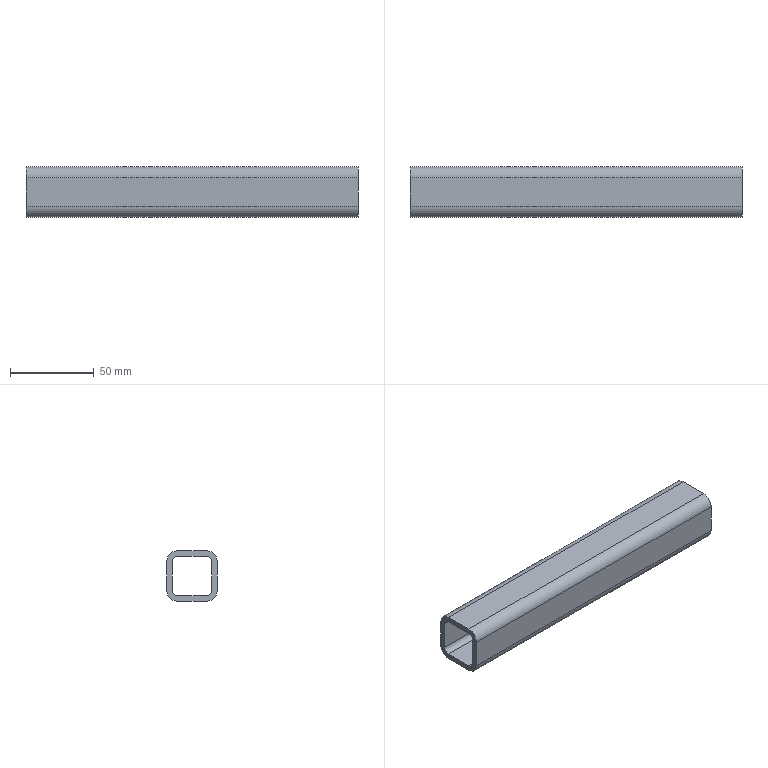Part | STEP file | [01]-7 | 1 solid | 18 faces | box 197.8 x 30 x 30 mm | volume 62637 mm3 | plane 10 | cylinder 8 | commonest cylinder face diameters 6.4 x4 12.8 x4
STEP:
#1=CARTESIAN_POINT('',(5.,23.6,0.));
#2=VERTEX_POINT('',#1);
#3=CARTESIAN_POINT('',(5.,30.,6.4));
#4=VERTEX_POINT('',#3);
#5=CARTESIAN_POINT('',(5.,23.6,6.4));
#6=DIRECTION('',(1.,0.,0.));
#7=DIRECTION('',(0.,0.,-1.));
#8=AXIS2_PLACEMENT_3D('',#5,#6,#7);
#9=CIRCLE('',#8,6.4);
#10=EDGE_CURVE('',#2,#4,#9,.T.);
#11=ORIENTED_EDGE('',*,*,#10,.T.);
#12=CARTESIAN_POINT('',(202.8,30.,6.4));
#13=VERTEX_POINT('',#12);
#14=CARTESIAN_POINT('',(202.8,30.,6.4));
#15=DIRECTION('',(-1.,0.,0.));
#16=VECTOR('',#15,1000.);
#17=LINE('',#14,#16);
#18=EDGE_CURVE('',#13,#4,#17,.T.);
#19=ORIENTED_EDGE('',*,*,#18,.F.);
#20=CARTESIAN_POINT('',(202.8,23.6,0.));
#21=VERTEX_POINT('',#20);
#22=CARTESIAN_POINT('',(202.8,23.6,6.4));
#23=DIRECTION('',(1.,0.,0.));
#24=DIRECTION('',(0.,0.,-1.));
#25=AXIS2_PLACEMENT_3D('',#22,#23,#24);
#26=CIRCLE('',#25,6.4);
#27=EDGE_CURVE('',#21,#13,#26,.T.);
#28=ORIENTED_EDGE('',*,*,#27,.F.);
#29=CARTESIAN_POINT('',(202.8,23.6,0.));
#30=DIRECTION('',(-1.,0.,0.));
#31=VECTOR('',#30,1000.);
#32=LINE('',#29,#31);
#33=EDGE_CURVE('',#21,#2,#32,.T.);
#34=ORIENTED_EDGE('',*,*,#33,.T.);
#35=EDGE_LOOP('',(#11,#19,#28,#34));
#36=FACE_OUTER_BOUND('',#35,.T.);
#37=CARTESIAN_POINT('',(202.8,23.6,6.4));
#38=DIRECTION('',(-1.,0.,0.));
#39=DIRECTION('',(0.,0.,1.));
#40=AXIS2_PLACEMENT_3D('',#37,#38,#39);
#41=CYLINDRICAL_SURFACE('',#40,6.4);
#42=ADVANCED_FACE('',(#36),#41,.T.);
#43=CARTESIAN_POINT('',(5.,30.,23.6));
#44=VERTEX_POINT('',#43);
#45=CARTESIAN_POINT('',(5.,30.,6.4));
#46=DIRECTION('',(0.,0.,1.));
#47=VECTOR('',#46,1000.);
#48=LINE('',#45,#47);
#49=EDGE_CURVE('',#4,#44,#48,.T.);
#50=ORIENTED_EDGE('',*,*,#49,.T.);
#51=CARTESIAN_POINT('',(202.8,30.,23.6));
#52=VERTEX_POINT('',#51);
#53=CARTESIAN_POINT('',(202.8,30.,23.6));
#54=DIRECTION('',(-1.,0.,0.));
#55=VECTOR('',#54,1000.);
#56=LINE('',#53,#55);
#57=EDGE_CURVE('',#52,#44,#56,.T.);
#58=ORIENTED_EDGE('',*,*,#57,.F.);
#59=CARTESIAN_POINT('',(202.8,30.,6.4));
#60=DIRECTION('',(0.,0.,1.));
#61=VECTOR('',#60,1000.);
#62=LINE('',#59,#61);
#63=EDGE_CURVE('',#13,#52,#62,.T.);
#64=ORIENTED_EDGE('',*,*,#63,.F.);
#65=ORIENTED_EDGE('',*,*,#18,.T.);
#66=EDGE_LOOP('',(#50,#58,#64,#65));
#67=FACE_OUTER_BOUND('',#66,.T.);
#68=CARTESIAN_POINT('',(202.8,30.,6.4));
#69=DIRECTION('',(0.,-1.,0.));
#70=DIRECTION('',(0.,0.,-1.));
#71=AXIS2_PLACEMENT_3D('',#68,#69,#70);
#72=PLANE('',#71);
#73=ADVANCED_FACE('',(#67),#72,.F.);
#74=CARTESIAN_POINT('',(5.,23.6,30.));
#75=VERTEX_POINT('',#74);
#76=CARTESIAN_POINT('',(5.,23.6,23.6));
#77=DIRECTION('',(1.,0.,0.));
#78=DIRECTION('',(0.,0.,-1.));
#79=AXIS2_PLACEMENT_3D('',#76,#77,#78);
#80=CIRCLE('',#79,6.4);
#81=EDGE_CURVE('',#44,#75,#80,.T.);
#82=ORIENTED_EDGE('',*,*,#81,.T.);
#83=CARTESIAN_POINT('',(202.8,23.6,30.));
#84=VERTEX_POINT('',#83);
#85=CARTESIAN_POINT('',(202.8,23.6,30.));
#86=DIRECTION('',(-1.,0.,0.));
#87=VECTOR('',#86,1000.);
#88=LINE('',#85,#87);
#89=EDGE_CURVE('',#84,#75,#88,.T.);
#90=ORIENTED_EDGE('',*,*,#89,.F.);
#91=CARTESIAN_POINT('',(202.8,23.6,23.6));
#92=DIRECTION('',(1.,0.,0.));
#93=DIRECTION('',(0.,0.,-1.));
#94=AXIS2_PLACEMENT_3D('',#91,#92,#93);
#95=CIRCLE('',#94,6.4);
#96=EDGE_CURVE('',#52,#84,#95,.T.);
#97=ORIENTED_EDGE('',*,*,#96,.F.);
#98=ORIENTED_EDGE('',*,*,#57,.T.);
#99=EDGE_LOOP('',(#82,#90,#97,#98));
#100=FACE_OUTER_BOUND('',#99,.T.);
#101=CARTESIAN_POINT('',(202.8,23.6,23.6));
#102=DIRECTION('',(-1.,0.,0.));
#103=DIRECTION('',(0.,0.,1.));
#104=AXIS2_PLACEMENT_3D('',#101,#102,#103);
#105=CYLINDRICAL_SURFACE('',#104,6.4);
#106=ADVANCED_FACE('',(#100),#105,.T.);
#107=CARTESIAN_POINT('',(5.,6.4,30.));
#108=VERTEX_POINT('',#107);
#109=CARTESIAN_POINT('',(5.,23.6,30.));
#110=DIRECTION('',(0.,-1.,0.));
#111=VECTOR('',#110,1000.);
#112=LINE('',#109,#111);
#113=EDGE_CURVE('',#75,#108,#112,.T.);
#114=ORIENTED_EDGE('',*,*,#113,.T.);
#115=CARTESIAN_POINT('',(202.8,6.4,30.));
#116=VERTEX_POINT('',#115);
#117=CARTESIAN_POINT('',(202.8,6.4,30.));
#118=DIRECTION('',(-1.,0.,0.));
#119=VECTOR('',#118,1000.);
#120=LINE('',#117,#119);
#121=EDGE_CURVE('',#116,#108,#120,.T.);
#122=ORIENTED_EDGE('',*,*,#121,.F.);
#123=CARTESIAN_POINT('',(202.8,23.6,30.));
#124=DIRECTION('',(0.,-1.,0.));
#125=VECTOR('',#124,1000.);
#126=LINE('',#123,#125);
#127=EDGE_CURVE('',#84,#116,#126,.T.);
#128=ORIENTED_EDGE('',*,*,#127,.F.);
#129=ORIENTED_EDGE('',*,*,#89,.T.);
#130=EDGE_LOOP('',(#114,#122,#128,#129));
#131=FACE_OUTER_BOUND('',#130,.T.);
#132=CARTESIAN_POINT('',(202.8,23.6,30.));
#133=DIRECTION('',(0.,0.,-1.));
#134=DIRECTION('',(0.,1.,0.));
#135=AXIS2_PLACEMENT_3D('',#132,#133,#134);
#136=PLANE('',#135);
#137=ADVANCED_FACE('',(#131),#136,.F.);
#138=CARTESIAN_POINT('',(5.,0.,23.6));
#139=VERTEX_POINT('',#138);
#140=CARTESIAN_POINT('',(5.,6.4,23.6));
#141=DIRECTION('',(1.,0.,0.));
#142=DIRECTION('',(0.,0.,-1.));
#143=AXIS2_PLACEMENT_3D('',#140,#141,#142);
#144=CIRCLE('',#143,6.4);
#145=EDGE_CURVE('',#108,#139,#144,.T.);
#146=ORIENTED_EDGE('',*,*,#145,.T.);
#147=CARTESIAN_POINT('',(202.8,0.,23.6));
#148=VERTEX_POINT('',#147);
#149=CARTESIAN_POINT('',(202.8,0.,23.6));
#150=DIRECTION('',(-1.,0.,0.));
#151=VECTOR('',#150,1000.);
#152=LINE('',#149,#151);
#153=EDGE_CURVE('',#148,#139,#152,.T.);
#154=ORIENTED_EDGE('',*,*,#153,.F.);
#155=CARTESIAN_POINT('',(202.8,6.4,23.6));
#156=DIRECTION('',(1.,0.,0.));
#157=DIRECTION('',(0.,0.,-1.));
#158=AXIS2_PLACEMENT_3D('',#155,#156,#157);
#159=CIRCLE('',#158,6.4);
#160=EDGE_CURVE('',#116,#148,#159,.T.);
#161=ORIENTED_EDGE('',*,*,#160,.F.);
#162=ORIENTED_EDGE('',*,*,#121,.T.);
#163=EDGE_LOOP('',(#146,#154,#161,#162));
#164=FACE_OUTER_BOUND('',#163,.T.);
#165=CARTESIAN_POINT('',(202.8,6.4,23.6));
#166=DIRECTION('',(-1.,0.,0.));
#167=DIRECTION('',(0.,0.,1.));
#168=AXIS2_PLACEMENT_3D('',#165,#166,#167);
#169=CYLINDRICAL_SURFACE('',#168,6.4);
#170=ADVANCED_FACE('',(#164),#169,.T.);
#171=CARTESIAN_POINT('',(5.,0.,6.4));
#172=VERTEX_POINT('',#171);
#173=CARTESIAN_POINT('',(5.,0.,23.6));
#174=DIRECTION('',(0.,0.,-1.));
#175=VECTOR('',#174,1000.);
#176=LINE('',#173,#175);
#177=EDGE_CURVE('',#139,#172,#176,.T.);
#178=ORIENTED_EDGE('',*,*,#177,.T.);
#179=CARTESIAN_POINT('',(202.8,0.,6.4));
#180=VERTEX_POINT('',#179);
#181=CARTESIAN_POINT('',(202.8,0.,6.4));
#182=DIRECTION('',(-1.,0.,0.));
#183=VECTOR('',#182,1000.);
#184=LINE('',#181,#183);
#185=EDGE_CURVE('',#180,#172,#184,.T.);
#186=ORIENTED_EDGE('',*,*,#185,.F.);
#187=CARTESIAN_POINT('',(202.8,0.,23.6));
#188=DIRECTION('',(0.,0.,-1.));
#189=VECTOR('',#188,1000.);
#190=LINE('',#187,#189);
#191=EDGE_CURVE('',#148,#180,#190,.T.);
#192=ORIENTED_EDGE('',*,*,#191,.F.);
#193=ORIENTED_EDGE('',*,*,#153,.T.);
#194=EDGE_LOOP('',(#178,#186,#192,#193));
#195=FACE_OUTER_BOUND('',#194,.T.);
#196=CARTESIAN_POINT('',(202.8,0.,23.6));
#197=DIRECTION('',(0.,1.,0.));
#198=DIRECTION('',(0.,0.,1.));
#199=AXIS2_PLACEMENT_3D('',#196,#197,#198);
#200=PLANE('',#199);
#201=ADVANCED_FACE('',(#195),#200,.F.);
#202=CARTESIAN_POINT('',(5.,6.4,0.));
#203=VERTEX_POINT('',#202);
#204=CARTESIAN_POINT('',(5.,6.4,6.4));
#205=DIRECTION('',(1.,0.,0.));
#206=DIRECTION('',(0.,0.,-1.));
#207=AXIS2_PLACEMENT_3D('',#204,#205,#206);
#208=CIRCLE('',#207,6.4);
#209=EDGE_CURVE('',#172,#203,#208,.T.);
#210=ORIENTED_EDGE('',*,*,#209,.T.);
#211=CARTESIAN_POINT('',(202.8,6.4,0.));
#212=VERTEX_POINT('',#211);
#213=CARTESIAN_POINT('',(202.8,6.4,0.));
#214=DIRECTION('',(-1.,0.,0.));
#215=VECTOR('',#214,1000.);
#216=LINE('',#213,#215);
#217=EDGE_CURVE('',#212,#203,#216,.T.);
#218=ORIENTED_EDGE('',*,*,#217,.F.);
#219=CARTESIAN_POINT('',(202.8,6.4,6.4));
#220=DIRECTION('',(1.,0.,0.));
#221=DIRECTION('',(0.,0.,-1.));
#222=AXIS2_PLACEMENT_3D('',#219,#220,#221);
#223=CIRCLE('',#222,6.4);
#224=EDGE_CURVE('',#180,#212,#223,.T.);
#225=ORIENTED_EDGE('',*,*,#224,.F.);
#226=ORIENTED_EDGE('',*,*,#185,.T.);
#227=EDGE_LOOP('',(#210,#218,#225,#226));
#228=FACE_OUTER_BOUND('',#227,.T.);
#229=CARTESIAN_POINT('',(202.8,6.4,6.4));
#230=DIRECTION('',(-1.,0.,0.));
#231=DIRECTION('',(0.,0.,1.));
#232=AXIS2_PLACEMENT_3D('',#229,#230,#231);
#233=CYLINDRICAL_SURFACE('',#232,6.4);
#234=ADVANCED_FACE('',(#228),#233,.T.);
#235=CARTESIAN_POINT('',(5.,6.4,0.));
#236=DIRECTION('',(0.,1.,0.));
#237=VECTOR('',#236,1000.);
#238=LINE('',#235,#237);
#239=EDGE_CURVE('',#203,#2,#238,.T.);
#240=ORIENTED_EDGE('',*,*,#239,.T.);
#241=ORIENTED_EDGE('',*,*,#33,.F.);
#242=CARTESIAN_POINT('',(202.8,6.4,0.));
#243=DIRECTION('',(0.,1.,0.));
#244=VECTOR('',#243,1000.);
#245=LINE('',#242,#244);
#246=EDGE_CURVE('',#212,#21,#245,.T.);
#247=ORIENTED_EDGE('',*,*,#246,.F.);
#248=ORIENTED_EDGE('',*,*,#217,.T.);
#249=EDGE_LOOP('',(#240,#241,#247,#248));
#250=FACE_OUTER_BOUND('',#249,.T.);
#251=CARTESIAN_POINT('',(202.8,6.4,0.));
#252=DIRECTION('',(0.,0.,1.));
#253=DIRECTION('',(0.,-1.,0.));
#254=AXIS2_PLACEMENT_3D('',#251,#252,#253);
#255=PLANE('',#254);
#256=ADVANCED_FACE('',(#250),#255,.F.);
#257=CARTESIAN_POINT('',(202.8,26.8,23.6));
#258=VERTEX_POINT('',#257);
#259=CARTESIAN_POINT('',(202.8,23.6,26.8));
#260=VERTEX_POINT('',#259);
#261=CARTESIAN_POINT('',(202.8,23.6,23.6));
#262=DIRECTION('',(1.,0.,0.));
#263=DIRECTION('',(0.,0.,-1.));
#264=AXIS2_PLACEMENT_3D('',#261,#262,#263);
#265=CIRCLE('',#264,3.2);
#266=EDGE_CURVE('',#258,#260,#265,.T.);
#267=ORIENTED_EDGE('',*,*,#266,.F.);
#268=CARTESIAN_POINT('',(202.8,26.8,6.4));
#269=VERTEX_POINT('',#268);
#270=CARTESIAN_POINT('',(202.8,26.8,6.4));
#271=DIRECTION('',(0.,0.,1.));
#272=VECTOR('',#271,1000.);
#273=LINE('',#270,#272);
#274=EDGE_CURVE('',#269,#258,#273,.T.);
#275=ORIENTED_EDGE('',*,*,#274,.F.);
#276=CARTESIAN_POINT('',(202.8,23.6,3.2));
#277=VERTEX_POINT('',#276);
#278=CARTESIAN_POINT('',(202.8,23.6,6.4));
#279=DIRECTION('',(1.,0.,0.));
#280=DIRECTION('',(0.,0.,-1.));
#281=AXIS2_PLACEMENT_3D('',#278,#279,#280);
#282=CIRCLE('',#281,3.2);
#283=EDGE_CURVE('',#277,#269,#282,.T.);
#284=ORIENTED_EDGE('',*,*,#283,.F.);
#285=CARTESIAN_POINT('',(202.8,6.4,3.2));
#286=VERTEX_POINT('',#285);
#287=CARTESIAN_POINT('',(202.8,6.4,3.2));
#288=DIRECTION('',(0.,1.,0.));
#289=VECTOR('',#288,1000.);
#290=LINE('',#287,#289);
#291=EDGE_CURVE('',#286,#277,#290,.T.);
#292=ORIENTED_EDGE('',*,*,#291,.F.);
#293=CARTESIAN_POINT('',(202.8,3.2,6.4));
#294=VERTEX_POINT('',#293);
#295=CARTESIAN_POINT('',(202.8,6.4,6.4));
#296=DIRECTION('',(1.,0.,0.));
#297=DIRECTION('',(0.,0.,-1.));
#298=AXIS2_PLACEMENT_3D('',#295,#296,#297);
#299=CIRCLE('',#298,3.2);
#300=EDGE_CURVE('',#294,#286,#299,.T.);
#301=ORIENTED_EDGE('',*,*,#300,.F.);
#302=CARTESIAN_POINT('',(202.8,3.2,23.6));
#303=VERTEX_POINT('',#302);
#304=CARTESIAN_POINT('',(202.8,3.2,23.6));
#305=DIRECTION('',(0.,0.,-1.));
#306=VECTOR('',#305,1000.);
#307=LINE('',#304,#306);
#308=EDGE_CURVE('',#303,#294,#307,.T.);
#309=ORIENTED_EDGE('',*,*,#308,.F.);
#310=CARTESIAN_POINT('',(202.8,6.4,26.8));
#311=VERTEX_POINT('',#310);
#312=CARTESIAN_POINT('',(202.8,6.4,23.6));
#313=DIRECTION('',(1.,0.,0.));
#314=DIRECTION('',(0.,0.,-1.));
#315=AXIS2_PLACEMENT_3D('',#312,#313,#314);
#316=CIRCLE('',#315,3.2);
#317=EDGE_CURVE('',#311,#303,#316,.T.);
#318=ORIENTED_EDGE('',*,*,#317,.F.);
#319=CARTESIAN_POINT('',(202.8,23.6,26.8));
#320=DIRECTION('',(0.,-1.,0.));
#321=VECTOR('',#320,1000.);
#322=LINE('',#319,#321);
#323=EDGE_CURVE('',#260,#311,#322,.T.);
#324=ORIENTED_EDGE('',*,*,#323,.F.);
#325=EDGE_LOOP('',(#267,#275,#284,#292,#301,#309,#318,#324));
#326=FACE_BOUND('',#325,.T.);
#327=ORIENTED_EDGE('',*,*,#27,.T.);
#328=ORIENTED_EDGE('',*,*,#63,.T.);
#329=ORIENTED_EDGE('',*,*,#96,.T.);
#330=ORIENTED_EDGE('',*,*,#127,.T.);
#331=ORIENTED_EDGE('',*,*,#160,.T.);
#332=ORIENTED_EDGE('',*,*,#191,.T.);
#333=ORIENTED_EDGE('',*,*,#224,.T.);
#334=ORIENTED_EDGE('',*,*,#246,.T.);
#335=EDGE_LOOP('',(#327,#328,#329,#330,#331,#332,#333,#334));
#336=FACE_OUTER_BOUND('',#335,.T.);
#337=CARTESIAN_POINT('',(202.8,23.6,6.4));
#338=DIRECTION('',(1.,0.,0.));
#339=DIRECTION('',(0.,0.,-1.));
#340=AXIS2_PLACEMENT_3D('',#337,#338,#339);
#341=PLANE('',#340);
#342=ADVANCED_FACE('',(#326,#336),#341,.T.);
#343=CARTESIAN_POINT('',(5.,26.8,6.4));
#344=VERTEX_POINT('',#343);
#345=CARTESIAN_POINT('',(5.,26.8,23.6));
#346=VERTEX_POINT('',#345);
#347=CARTESIAN_POINT('',(5.,26.8,6.4));
#348=DIRECTION('',(0.,0.,1.));
#349=VECTOR('',#348,1000.);
#350=LINE('',#347,#349);
#351=EDGE_CURVE('',#344,#346,#350,.T.);
#352=ORIENTED_EDGE('',*,*,#351,.T.);
#353=CARTESIAN_POINT('',(5.,23.6,26.8));
#354=VERTEX_POINT('',#353);
#355=CARTESIAN_POINT('',(5.,23.6,23.6));
#356=DIRECTION('',(1.,0.,0.));
#357=DIRECTION('',(0.,0.,-1.));
#358=AXIS2_PLACEMENT_3D('',#355,#356,#357);
#359=CIRCLE('',#358,3.2);
#360=EDGE_CURVE('',#346,#354,#359,.T.);
#361=ORIENTED_EDGE('',*,*,#360,.T.);
#362=CARTESIAN_POINT('',(5.,6.4,26.8));
#363=VERTEX_POINT('',#362);
#364=CARTESIAN_POINT('',(5.,23.6,26.8));
#365=DIRECTION('',(0.,-1.,0.));
#366=VECTOR('',#365,1000.);
#367=LINE('',#364,#366);
#368=EDGE_CURVE('',#354,#363,#367,.T.);
#369=ORIENTED_EDGE('',*,*,#368,.T.);
#370=CARTESIAN_POINT('',(5.,3.2,23.6));
#371=VERTEX_POINT('',#370);
#372=CARTESIAN_POINT('',(5.,6.4,23.6));
#373=DIRECTION('',(1.,0.,0.));
#374=DIRECTION('',(0.,0.,-1.));
#375=AXIS2_PLACEMENT_3D('',#372,#373,#374);
#376=CIRCLE('',#375,3.2);
#377=EDGE_CURVE('',#363,#371,#376,.T.);
#378=ORIENTED_EDGE('',*,*,#377,.T.);
#379=CARTESIAN_POINT('',(5.,3.2,6.4));
#380=VERTEX_POINT('',#379);
#381=CARTESIAN_POINT('',(5.,3.2,23.6));
#382=DIRECTION('',(0.,0.,-1.));
#383=VECTOR('',#382,1000.);
#384=LINE('',#381,#383);
#385=EDGE_CURVE('',#371,#380,#384,.T.);
#386=ORIENTED_EDGE('',*,*,#385,.T.);
#387=CARTESIAN_POINT('',(5.,6.4,3.2));
#388=VERTEX_POINT('',#387);
#389=CARTESIAN_POINT('',(5.,6.4,6.4));
#390=DIRECTION('',(1.,0.,0.));
#391=DIRECTION('',(0.,0.,-1.));
#392=AXIS2_PLACEMENT_3D('',#389,#390,#391);
#393=CIRCLE('',#392,3.2);
#394=EDGE_CURVE('',#380,#388,#393,.T.);
#395=ORIENTED_EDGE('',*,*,#394,.T.);
#396=CARTESIAN_POINT('',(5.,23.6,3.2));
#397=VERTEX_POINT('',#396);
#398=CARTESIAN_POINT('',(5.,6.4,3.2));
#399=DIRECTION('',(0.,1.,0.));
#400=VECTOR('',#399,1000.);
#401=LINE('',#398,#400);
#402=EDGE_CURVE('',#388,#397,#401,.T.);
#403=ORIENTED_EDGE('',*,*,#402,.T.);
#404=CARTESIAN_POINT('',(5.,23.6,6.4));
#405=DIRECTION('',(1.,0.,0.));
#406=DIRECTION('',(0.,0.,-1.));
#407=AXIS2_PLACEMENT_3D('',#404,#405,#406);
#408=CIRCLE('',#407,3.2);
#409=EDGE_CURVE('',#397,#344,#408,.T.);
#410=ORIENTED_EDGE('',*,*,#409,.T.);
#411=EDGE_LOOP('',(#352,#361,#369,#378,#386,#395,#403,#410));
#412=FACE_BOUND('',#411,.T.);
#413=ORIENTED_EDGE('',*,*,#10,.F.);
#414=ORIENTED_EDGE('',*,*,#239,.F.);
#415=ORIENTED_EDGE('',*,*,#209,.F.);
#416=ORIENTED_EDGE('',*,*,#177,.F.);
#417=ORIENTED_EDGE('',*,*,#145,.F.);
#418=ORIENTED_EDGE('',*,*,#113,.F.);
#419=ORIENTED_EDGE('',*,*,#81,.F.);
#420=ORIENTED_EDGE('',*,*,#49,.F.);
#421=EDGE_LOOP('',(#413,#414,#415,#416,#417,#418,#419,#420));
#422=FACE_OUTER_BOUND('',#421,.T.);
#423=CARTESIAN_POINT('',(5.,23.6,6.4));
#424=DIRECTION('',(1.,0.,0.));
#425=DIRECTION('',(0.,0.,-1.));
#426=AXIS2_PLACEMENT_3D('',#423,#424,#425);
#427=PLANE('',#426);
#428=ADVANCED_FACE('',(#412,#422),#427,.F.);
#429=ORIENTED_EDGE('',*,*,#351,.F.);
#430=CARTESIAN_POINT('',(202.8,26.8,6.4));
#431=DIRECTION('',(-1.,0.,0.));
#432=VECTOR('',#431,1000.);
#433=LINE('',#430,#432);
#434=EDGE_CURVE('',#269,#344,#433,.T.);
#435=ORIENTED_EDGE('',*,*,#434,.F.);
#436=ORIENTED_EDGE('',*,*,#274,.T.);
#437=CARTESIAN_POINT('',(202.8,26.8,23.6));
#438=DIRECTION('',(-1.,0.,0.));
#439=VECTOR('',#438,1000.);
#440=LINE('',#437,#439);
#441=EDGE_CURVE('',#258,#346,#440,.T.);
#442=ORIENTED_EDGE('',*,*,#441,.T.);
#443=EDGE_LOOP('',(#429,#435,#436,#442));
#444=FACE_OUTER_BOUND('',#443,.T.);
#445=CARTESIAN_POINT('',(202.8,26.8,6.4));
#446=DIRECTION('',(0.,-1.,0.));
#447=DIRECTION('',(-1.,0.,0.));
#448=AXIS2_PLACEMENT_3D('',#445,#446,#447);
#449=PLANE('',#448);
#450=ADVANCED_FACE('',(#444),#449,.T.);
#451=ORIENTED_EDGE('',*,*,#360,.F.);
#452=ORIENTED_EDGE('',*,*,#441,.F.);
#453=ORIENTED_EDGE('',*,*,#266,.T.);
#454=CARTESIAN_POINT('',(202.8,23.6,26.8));
#455=DIRECTION('',(-1.,0.,0.));
#456=VECTOR('',#455,1000.);
#457=LINE('',#454,#456);
#458=EDGE_CURVE('',#260,#354,#457,.T.);
#459=ORIENTED_EDGE('',*,*,#458,.T.);
#460=EDGE_LOOP('',(#451,#452,#453,#459));
#461=FACE_OUTER_BOUND('',#460,.T.);
#462=CARTESIAN_POINT('',(202.8,23.6,23.6));
#463=DIRECTION('',(-1.,0.,0.));
#464=DIRECTION('',(0.,0.,1.));
#465=AXIS2_PLACEMENT_3D('',#462,#463,#464);
#466=CYLINDRICAL_SURFACE('',#465,3.2);
#467=ADVANCED_FACE('',(#461),#466,.F.);
#468=ORIENTED_EDGE('',*,*,#368,.F.);
#469=ORIENTED_EDGE('',*,*,#458,.F.);
#470=ORIENTED_EDGE('',*,*,#323,.T.);
#471=CARTESIAN_POINT('',(202.8,6.4,26.8));
#472=DIRECTION('',(-1.,0.,0.));
#473=VECTOR('',#472,1000.);
#474=LINE('',#471,#473);
#475=EDGE_CURVE('',#311,#363,#474,.T.);
#476=ORIENTED_EDGE('',*,*,#475,.T.);
#477=EDGE_LOOP('',(#468,#469,#470,#476));
#478=FACE_OUTER_BOUND('',#477,.T.);
#479=CARTESIAN_POINT('',(202.8,23.6,26.8));
#480=DIRECTION('',(0.,0.,-1.));
#481=DIRECTION('',(-1.,0.,0.));
#482=AXIS2_PLACEMENT_3D('',#479,#480,#481);
#483=PLANE('',#482);
#484=ADVANCED_FACE('',(#478),#483,.T.);
#485=ORIENTED_EDGE('',*,*,#377,.F.);
#486=ORIENTED_EDGE('',*,*,#475,.F.);
#487=ORIENTED_EDGE('',*,*,#317,.T.);
#488=CARTESIAN_POINT('',(202.8,3.2,23.6));
#489=DIRECTION('',(-1.,0.,0.));
#490=VECTOR('',#489,1000.);
#491=LINE('',#488,#490);
#492=EDGE_CURVE('',#303,#371,#491,.T.);
#493=ORIENTED_EDGE('',*,*,#492,.T.);
#494=EDGE_LOOP('',(#485,#486,#487,#493));
#495=FACE_OUTER_BOUND('',#494,.T.);
#496=CARTESIAN_POINT('',(202.8,6.4,23.6));
#497=DIRECTION('',(-1.,0.,0.));
#498=DIRECTION('',(0.,0.,1.));
#499=AXIS2_PLACEMENT_3D('',#496,#497,#498);
#500=CYLINDRICAL_SURFACE('',#499,3.2);
#501=ADVANCED_FACE('',(#495),#500,.F.);
#502=ORIENTED_EDGE('',*,*,#385,.F.);
#503=ORIENTED_EDGE('',*,*,#492,.F.);
#504=ORIENTED_EDGE('',*,*,#308,.T.);
#505=CARTESIAN_POINT('',(202.8,3.2,6.4));
#506=DIRECTION('',(-1.,0.,0.));
#507=VECTOR('',#506,1000.);
#508=LINE('',#505,#507);
#509=EDGE_CURVE('',#294,#380,#508,.T.);
#510=ORIENTED_EDGE('',*,*,#509,.T.);
#511=EDGE_LOOP('',(#502,#503,#504,#510));
#512=FACE_OUTER_BOUND('',#511,.T.);
#513=CARTESIAN_POINT('',(202.8,3.2,23.6));
#514=DIRECTION('',(0.,1.,0.));
#515=DIRECTION('',(1.,0.,0.));
#516=AXIS2_PLACEMENT_3D('',#513,#514,#515);
#517=PLANE('',#516);
#518=ADVANCED_FACE('',(#512),#517,.T.);
#519=ORIENTED_EDGE('',*,*,#394,.F.);
#520=ORIENTED_EDGE('',*,*,#509,.F.);
#521=ORIENTED_EDGE('',*,*,#300,.T.);
#522=CARTESIAN_POINT('',(202.8,6.4,3.2));
#523=DIRECTION('',(-1.,0.,0.));
#524=VECTOR('',#523,1000.);
#525=LINE('',#522,#524);
#526=EDGE_CURVE('',#286,#388,#525,.T.);
#527=ORIENTED_EDGE('',*,*,#526,.T.);
#528=EDGE_LOOP('',(#519,#520,#521,#527));
#529=FACE_OUTER_BOUND('',#528,.T.);
#530=CARTESIAN_POINT('',(202.8,6.4,6.4));
#531=DIRECTION('',(-1.,0.,0.));
#532=DIRECTION('',(0.,0.,1.));
#533=AXIS2_PLACEMENT_3D('',#530,#531,#532);
#534=CYLINDRICAL_SURFACE('',#533,3.2);
#535=ADVANCED_FACE('',(#529),#534,.F.);
#536=ORIENTED_EDGE('',*,*,#402,.F.);
#537=ORIENTED_EDGE('',*,*,#526,.F.);
#538=ORIENTED_EDGE('',*,*,#291,.T.);
#539=CARTESIAN_POINT('',(202.8,23.6,3.2));
#540=DIRECTION('',(-1.,0.,0.));
#541=VECTOR('',#540,1000.);
#542=LINE('',#539,#541);
#543=EDGE_CURVE('',#277,#397,#542,.T.);
#544=ORIENTED_EDGE('',*,*,#543,.T.);
#545=EDGE_LOOP('',(#536,#537,#538,#544));
#546=FACE_OUTER_BOUND('',#545,.T.);
#547=CARTESIAN_POINT('',(202.8,6.4,3.2));
#548=DIRECTION('',(0.,0.,1.));
#549=DIRECTION('',(1.,0.,0.));
#550=AXIS2_PLACEMENT_3D('',#547,#548,#549);
#551=PLANE('',#550);
#552=ADVANCED_FACE('',(#546),#551,.T.);
#553=ORIENTED_EDGE('',*,*,#409,.F.);
#554=ORIENTED_EDGE('',*,*,#543,.F.);
#555=ORIENTED_EDGE('',*,*,#283,.T.);
#556=ORIENTED_EDGE('',*,*,#434,.T.);
#557=EDGE_LOOP('',(#553,#554,#555,#556));
#558=FACE_OUTER_BOUND('',#557,.T.);
#559=CARTESIAN_POINT('',(202.8,23.6,6.4));
#560=DIRECTION('',(-1.,0.,0.));
#561=DIRECTION('',(0.,0.,1.));
#562=AXIS2_PLACEMENT_3D('',#559,#560,#561);
#563=CYLINDRICAL_SURFACE('',#562,3.2);
#564=ADVANCED_FACE('',(#558),#563,.F.);
#565=CLOSED_SHELL('',(#42,#73,#106,#137,#170,#201,#234,#256,#342,#428,#450,#467,#484,#501,#518,#535,#552,#564));
#566=MANIFOLD_SOLID_BREP('',#565);
#567=CARTESIAN_POINT('',(0.,0.,0.));
#568=DIRECTION('',(0.,0.,1.));
#569=DIRECTION('',(1.,0.,0.));
#570=AXIS2_PLACEMENT_3D('',#567,#568,#569);
#571=(LENGTH_UNIT()NAMED_UNIT(*)SI_UNIT(.MILLI.,.METRE.));
#572=UNCERTAINTY_MEASURE_WITH_UNIT(LENGTH_MEASURE(0.00001),#571,'','');
#573=(NAMED_UNIT(*)PLANE_ANGLE_UNIT()SI_UNIT($,.RADIAN.));
#574=(NAMED_UNIT(*)SI_UNIT($,.STERADIAN.)SOLID_ANGLE_UNIT());
#575=(GEOMETRIC_REPRESENTATION_CONTEXT(3)GLOBAL_UNCERTAINTY_ASSIGNED_CONTEXT((#572))GLOBAL_UNIT_ASSIGNED_CONTEXT((#571,#573,#574))REPRESENTATION_CONTEXT('',''));
#576=ADVANCED_BREP_SHAPE_REPRESENTATION('',(#566,#570),#575);